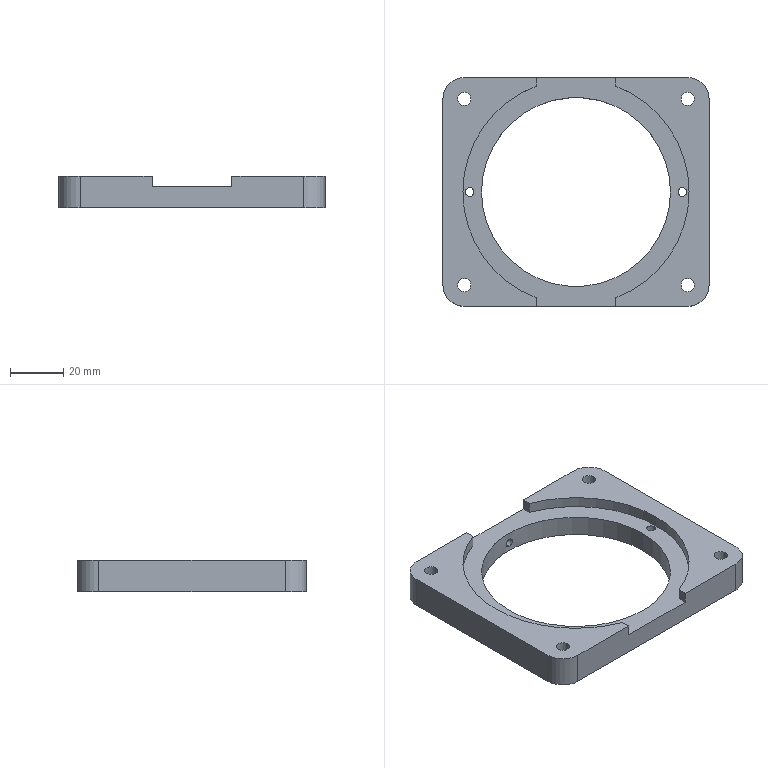Part | STEP file | QA-TE03 | 1 solid | 37 faces | box 100 x 86 x 12 mm | volume 46511 mm3 | cylinder 23 | plane 12 | cone 2 | commonest cylinder face diameters 5 x8 3.3 x6 16 x4 85 x3 71 x2